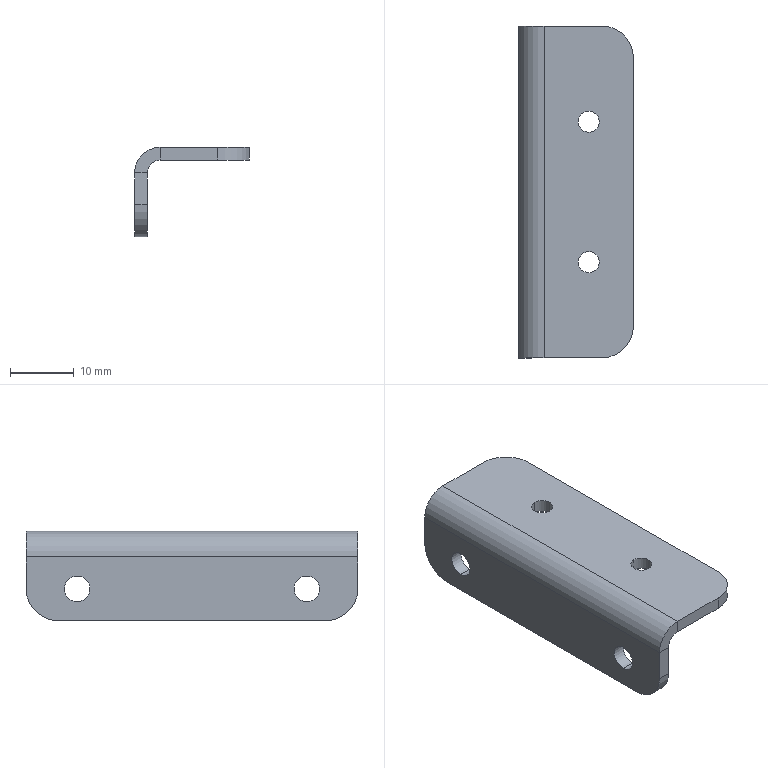Part | NX | features 镜向1 2 | 1 solid | 26 faces | box 18 x 52 x 14 mm | volume 2859 mm3 | cylinder 14 | plane 12 | commonest cylinder face diameters 4 x5 3.3 x4 10 x4 8 x1
STEP:
#1=CARTESIAN_POINT('',(50.,117.,-101.5));
#2=VERTEX_POINT('',#1);
#3=CARTESIAN_POINT('',(50.,117.,-105.5));
#4=VERTEX_POINT('',#3);
#5=CARTESIAN_POINT('',(50.,117.,-103.5));
#6=DIRECTION('',(-1.,0.,0.));
#7=DIRECTION('',(0.,0.,-1.));
#8=AXIS2_PLACEMENT_3D('',#5,#6,#7);
#9=CIRCLE('',#8,2.);
#10=EDGE_CURVE('',#2,#4,#9,.T.);
#11=ORIENTED_EDGE('',*,*,#10,.T.);
#12=CARTESIAN_POINT('',(52.,117.,-105.5));
#13=VERTEX_POINT('',#12);
#14=CARTESIAN_POINT('',(50.,117.,-105.5));
#15=DIRECTION('',(1.,0.,0.));
#16=VECTOR('',#15,1000.);
#17=LINE('',#14,#16);
#18=EDGE_CURVE('',#4,#13,#17,.T.);
#19=ORIENTED_EDGE('',*,*,#18,.T.);
#20=CARTESIAN_POINT('',(52.,117.,-101.5));
#21=VERTEX_POINT('',#20);
#22=CARTESIAN_POINT('',(52.,117.,-103.5));
#23=DIRECTION('',(-1.,0.,0.));
#24=DIRECTION('',(0.,0.,-1.));
#25=AXIS2_PLACEMENT_3D('',#22,#23,#24);
#26=CIRCLE('',#25,2.);
#27=EDGE_CURVE('',#21,#13,#26,.T.);
#28=ORIENTED_EDGE('',*,*,#27,.F.);
#29=CARTESIAN_POINT('',(50.,117.,-101.5));
#30=DIRECTION('',(1.,0.,0.));
#31=VECTOR('',#30,1000.);
#32=LINE('',#29,#31);
#33=EDGE_CURVE('',#21,#2,#32,.F.);
#34=ORIENTED_EDGE('',*,*,#33,.T.);
#35=EDGE_LOOP('',(#11,#19,#28,#34));
#36=FACE_BOUND('',#35,.T.);
#37=CARTESIAN_POINT('',(50.,117.,-103.5));
#38=DIRECTION('',(1.,0.,0.));
#39=DIRECTION('',(0.,0.,-1.));
#40=AXIS2_PLACEMENT_3D('',#37,#38,#39);
#41=CYLINDRICAL_SURFACE('',#40,2.);
#42=ADVANCED_FACE('',(#36),#41,.F.);
#43=CARTESIAN_POINT('',(50.,81.,-101.5));
#44=VERTEX_POINT('',#43);
#45=CARTESIAN_POINT('',(50.,81.,-105.5));
#46=VERTEX_POINT('',#45);
#47=CARTESIAN_POINT('',(50.,81.,-103.5));
#48=DIRECTION('',(-1.,0.,0.));
#49=DIRECTION('',(0.,0.,1.));
#50=AXIS2_PLACEMENT_3D('',#47,#48,#49);
#51=CIRCLE('',#50,2.);
#52=EDGE_CURVE('',#44,#46,#51,.T.);
#53=ORIENTED_EDGE('',*,*,#52,.T.);
#54=CARTESIAN_POINT('',(52.,81.,-105.5));
#55=VERTEX_POINT('',#54);
#56=CARTESIAN_POINT('',(50.,81.,-105.5));
#57=DIRECTION('',(1.,0.,0.));
#58=VECTOR('',#57,1000.);
#59=LINE('',#56,#58);
#60=EDGE_CURVE('',#55,#46,#59,.F.);
#61=ORIENTED_EDGE('',*,*,#60,.F.);
#62=CARTESIAN_POINT('',(52.,81.,-101.5));
#63=VERTEX_POINT('',#62);
#64=CARTESIAN_POINT('',(52.,81.,-103.5));
#65=DIRECTION('',(-1.,0.,0.));
#66=DIRECTION('',(0.,0.,1.));
#67=AXIS2_PLACEMENT_3D('',#64,#65,#66);
#68=CIRCLE('',#67,2.);
#69=EDGE_CURVE('',#63,#55,#68,.T.);
#70=ORIENTED_EDGE('',*,*,#69,.F.);
#71=CARTESIAN_POINT('',(50.,81.,-101.5));
#72=DIRECTION('',(1.,0.,0.));
#73=VECTOR('',#72,1000.);
#74=LINE('',#71,#73);
#75=EDGE_CURVE('',#44,#63,#74,.T.);
#76=ORIENTED_EDGE('',*,*,#75,.F.);
#77=EDGE_LOOP('',(#53,#61,#70,#76));
#78=FACE_BOUND('',#77,.T.);
#79=CARTESIAN_POINT('',(50.,81.,-103.5));
#80=DIRECTION('',(1.,0.,0.));
#81=DIRECTION('',(0.,0.,-1.));
#82=AXIS2_PLACEMENT_3D('',#79,#80,#81);
#83=CYLINDRICAL_SURFACE('',#82,2.);
#84=ADVANCED_FACE('',(#78),#83,.F.);
#85=CARTESIAN_POINT('',(61.,86.35,-96.5));
#86=VERTEX_POINT('',#85);
#87=CARTESIAN_POINT('',(61.,89.65,-96.5));
#88=VERTEX_POINT('',#87);
#89=CARTESIAN_POINT('',(61.,88.,-96.5));
#90=DIRECTION('',(0.,0.,1.));
#91=DIRECTION('',(0.,-1.,0.));
#92=AXIS2_PLACEMENT_3D('',#89,#90,#91);
#93=CIRCLE('',#92,1.65);
#94=EDGE_CURVE('',#86,#88,#93,.T.);
#95=ORIENTED_EDGE('',*,*,#94,.F.);
#96=CARTESIAN_POINT('',(61.,86.35,-94.5));
#97=VERTEX_POINT('',#96);
#98=CARTESIAN_POINT('',(61.,86.35,-94.5));
#99=DIRECTION('',(0.,0.,1.));
#100=VECTOR('',#99,1000.);
#101=LINE('',#98,#100);
#102=EDGE_CURVE('',#97,#86,#101,.F.);
#103=ORIENTED_EDGE('',*,*,#102,.F.);
#104=CARTESIAN_POINT('',(61.,89.65,-94.5));
#105=VERTEX_POINT('',#104);
#106=CARTESIAN_POINT('',(61.,88.,-94.5));
#107=DIRECTION('',(0.,0.,-1.));
#108=DIRECTION('',(0.,1.,0.));
#109=AXIS2_PLACEMENT_3D('',#106,#107,#108);
#110=CIRCLE('',#109,1.65);
#111=EDGE_CURVE('',#105,#97,#110,.T.);
#112=ORIENTED_EDGE('',*,*,#111,.F.);
#113=CARTESIAN_POINT('',(61.,89.65,-94.5));
#114=DIRECTION('',(0.,0.,1.));
#115=VECTOR('',#114,1000.);
#116=LINE('',#113,#115);
#117=EDGE_CURVE('',#88,#105,#116,.T.);
#118=ORIENTED_EDGE('',*,*,#117,.F.);
#119=EDGE_LOOP('',(#95,#103,#112,#118));
#120=FACE_BOUND('',#119,.T.);
#121=CARTESIAN_POINT('',(61.,88.,-94.5));
#122=DIRECTION('',(0.,0.,1.));
#123=DIRECTION('',(0.,-1.,0.));
#124=AXIS2_PLACEMENT_3D('',#121,#122,#123);
#125=CYLINDRICAL_SURFACE('',#124,1.65);
#126=ADVANCED_FACE('',(#120),#125,.F.);
#127=CARTESIAN_POINT('',(61.,108.35,-96.5));
#128=VERTEX_POINT('',#127);
#129=CARTESIAN_POINT('',(61.,111.65,-96.5));
#130=VERTEX_POINT('',#129);
#131=CARTESIAN_POINT('',(61.,110.,-96.5));
#132=DIRECTION('',(0.,0.,1.));
#133=DIRECTION('',(0.,-1.,0.));
#134=AXIS2_PLACEMENT_3D('',#131,#132,#133);
#135=CIRCLE('',#134,1.65);
#136=EDGE_CURVE('',#128,#130,#135,.T.);
#137=ORIENTED_EDGE('',*,*,#136,.F.);
#138=CARTESIAN_POINT('',(61.,108.35,-94.5));
#139=VERTEX_POINT('',#138);
#140=CARTESIAN_POINT('',(61.,108.35,-94.5));
#141=DIRECTION('',(0.,0.,1.));
#142=VECTOR('',#141,1000.);
#143=LINE('',#140,#142);
#144=EDGE_CURVE('',#139,#128,#143,.F.);
#145=ORIENTED_EDGE('',*,*,#144,.F.);
#146=CARTESIAN_POINT('',(61.,111.65,-94.5));
#147=VERTEX_POINT('',#146);
#148=CARTESIAN_POINT('',(61.,110.,-94.5));
#149=DIRECTION('',(0.,0.,-1.));
#150=DIRECTION('',(0.,1.,0.));
#151=AXIS2_PLACEMENT_3D('',#148,#149,#150);
#152=CIRCLE('',#151,1.65);
#153=EDGE_CURVE('',#147,#139,#152,.T.);
#154=ORIENTED_EDGE('',*,*,#153,.F.);
#155=CARTESIAN_POINT('',(61.,111.65,-94.5));
#156=DIRECTION('',(0.,0.,1.));
#157=VECTOR('',#156,1000.);
#158=LINE('',#155,#157);
#159=EDGE_CURVE('',#130,#147,#158,.T.);
#160=ORIENTED_EDGE('',*,*,#159,.F.);
#161=EDGE_LOOP('',(#137,#145,#154,#160));
#162=FACE_BOUND('',#161,.T.);
#163=CARTESIAN_POINT('',(61.,110.,-94.5));
#164=DIRECTION('',(0.,0.,1.));
#165=DIRECTION('',(0.,-1.,0.));
#166=AXIS2_PLACEMENT_3D('',#163,#164,#165);
#167=CYLINDRICAL_SURFACE('',#166,1.65);
#168=ADVANCED_FACE('',(#162),#167,.F.);
#169=ORIENTED_EDGE('',*,*,#111,.T.);
#170=CARTESIAN_POINT('',(61.,88.,-94.5));
#171=DIRECTION('',(0.,0.,-1.));
#172=DIRECTION('',(0.,1.,0.));
#173=AXIS2_PLACEMENT_3D('',#170,#171,#172);
#174=CIRCLE('',#173,1.65);
#175=EDGE_CURVE('',#97,#105,#174,.T.);
#176=ORIENTED_EDGE('',*,*,#175,.T.);
#177=EDGE_LOOP('',(#169,#176));
#178=FACE_BOUND('',#177,.T.);
#179=CARTESIAN_POINT('',(63.,125.,-94.5));
#180=VERTEX_POINT('',#179);
#181=CARTESIAN_POINT('',(54.,125.,-94.5));
#182=VERTEX_POINT('',#181);
#183=CARTESIAN_POINT('',(68.,125.,-94.5));
#184=DIRECTION('',(-1.,0.,0.));
#185=VECTOR('',#184,1000.);
#186=LINE('',#183,#185);
#187=EDGE_CURVE('',#180,#182,#186,.T.);
#188=ORIENTED_EDGE('',*,*,#187,.T.);
#189=CARTESIAN_POINT('',(54.,73.,-94.5));
#190=VERTEX_POINT('',#189);
#191=CARTESIAN_POINT('',(54.,125.,-94.5));
#192=DIRECTION('',(0.,-1.,0.));
#193=VECTOR('',#192,1000.);
#194=LINE('',#191,#193);
#195=EDGE_CURVE('',#182,#190,#194,.T.);
#196=ORIENTED_EDGE('',*,*,#195,.T.);
#197=CARTESIAN_POINT('',(63.,73.,-94.5));
#198=VERTEX_POINT('',#197);
#199=CARTESIAN_POINT('',(68.,73.,-94.5));
#200=DIRECTION('',(-1.,0.,0.));
#201=VECTOR('',#200,1000.);
#202=LINE('',#199,#201);
#203=EDGE_CURVE('',#198,#190,#202,.T.);
#204=ORIENTED_EDGE('',*,*,#203,.F.);
#205=CARTESIAN_POINT('',(68.,78.,-94.5));
#206=VERTEX_POINT('',#205);
#207=CARTESIAN_POINT('',(63.,78.,-94.5));
#208=DIRECTION('',(0.,0.,-1.));
#209=DIRECTION('',(0.,-1.,0.));
#210=AXIS2_PLACEMENT_3D('',#207,#208,#209);
#211=CIRCLE('',#210,5.);
#212=EDGE_CURVE('',#206,#198,#211,.T.);
#213=ORIENTED_EDGE('',*,*,#212,.F.);
#214=CARTESIAN_POINT('',(68.,120.,-94.5));
#215=VERTEX_POINT('',#214);
#216=CARTESIAN_POINT('',(68.,125.,-94.5));
#217=DIRECTION('',(0.,-1.,0.));
#218=VECTOR('',#217,1000.);
#219=LINE('',#216,#218);
#220=EDGE_CURVE('',#215,#206,#219,.T.);
#221=ORIENTED_EDGE('',*,*,#220,.F.);
#222=CARTESIAN_POINT('',(63.,120.,-94.5));
#223=DIRECTION('',(0.,0.,-1.));
#224=DIRECTION('',(0.,-1.,0.));
#225=AXIS2_PLACEMENT_3D('',#222,#223,#224);
#226=CIRCLE('',#225,5.);
#227=EDGE_CURVE('',#180,#215,#226,.T.);
#228=ORIENTED_EDGE('',*,*,#227,.F.);
#229=EDGE_LOOP('',(#188,#196,#204,#213,#221,#228));
#230=FACE_BOUND('',#229,.T.);
#231=ORIENTED_EDGE('',*,*,#153,.T.);
#232=CARTESIAN_POINT('',(61.,110.,-94.5));
#233=DIRECTION('',(0.,0.,-1.));
#234=DIRECTION('',(0.,1.,0.));
#235=AXIS2_PLACEMENT_3D('',#232,#233,#234);
#236=CIRCLE('',#235,1.65);
#237=EDGE_CURVE('',#139,#147,#236,.T.);
#238=ORIENTED_EDGE('',*,*,#237,.T.);
#239=EDGE_LOOP('',(#231,#238));
#240=FACE_BOUND('',#239,.T.);
#241=CARTESIAN_POINT('',(68.,125.,-94.5));
#242=DIRECTION('',(0.,0.,-1.));
#243=DIRECTION('',(0.,1.,0.));
#244=AXIS2_PLACEMENT_3D('',#241,#242,#243);
#245=PLANE('',#244);
#246=ADVANCED_FACE('',(#178,#230,#240),#245,.F.);
#247=CARTESIAN_POINT('',(54.,125.,-96.5));
#248=VERTEX_POINT('',#247);
#249=CARTESIAN_POINT('',(54.,125.,-94.5));
#250=DIRECTION('',(0.,0.,-1.));
#251=VECTOR('',#250,1000.);
#252=LINE('',#249,#251);
#253=EDGE_CURVE('',#182,#248,#252,.T.);
#254=ORIENTED_EDGE('',*,*,#253,.T.);
#255=CARTESIAN_POINT('',(52.,125.,-98.5));
#256=VERTEX_POINT('',#255);
#257=CARTESIAN_POINT('',(54.,125.,-98.5));
#258=DIRECTION('',(0.,-1.,0.));
#259=DIRECTION('',(0.,0.,-1.));
#260=AXIS2_PLACEMENT_3D('',#257,#258,#259);
#261=CIRCLE('',#260,2.);
#262=EDGE_CURVE('',#248,#256,#261,.T.);
#263=ORIENTED_EDGE('',*,*,#262,.T.);
#264=CARTESIAN_POINT('',(50.,125.,-98.5));
#265=VERTEX_POINT('',#264);
#266=CARTESIAN_POINT('',(52.,125.,-98.5));
#267=DIRECTION('',(-1.,0.,0.));
#268=VECTOR('',#267,1000.);
#269=LINE('',#266,#268);
#270=EDGE_CURVE('',#256,#265,#269,.T.);
#271=ORIENTED_EDGE('',*,*,#270,.T.);
#272=CARTESIAN_POINT('',(54.,125.,-98.5));
#273=DIRECTION('',(0.,-1.,0.));
#274=DIRECTION('',(0.,0.,1.));
#275=AXIS2_PLACEMENT_3D('',#272,#273,#274);
#276=CIRCLE('',#275,4.);
#277=EDGE_CURVE('',#182,#265,#276,.T.);
#278=ORIENTED_EDGE('',*,*,#277,.F.);
#279=EDGE_LOOP('',(#254,#263,#271,#278));
#280=FACE_BOUND('',#279,.T.);
#281=CARTESIAN_POINT('',(54.,125.,-94.5));
#282=DIRECTION('',(0.,1.,0.));
#283=DIRECTION('',(0.,0.,1.));
#284=AXIS2_PLACEMENT_3D('',#281,#282,#283);
#285=PLANE('',#284);
#286=ADVANCED_FACE('',(#280),#285,.T.);
#287=CARTESIAN_POINT('',(63.,125.,-96.5));
#288=VERTEX_POINT('',#287);
#289=CARTESIAN_POINT('',(68.,125.,-96.5));
#290=DIRECTION('',(-1.,0.,0.));
#291=VECTOR('',#290,1000.);
#292=LINE('',#289,#291);
#293=EDGE_CURVE('',#288,#248,#292,.T.);
#294=ORIENTED_EDGE('',*,*,#293,.T.);
#295=ORIENTED_EDGE('',*,*,#253,.F.);
#296=ORIENTED_EDGE('',*,*,#187,.F.);
#297=CARTESIAN_POINT('',(63.,125.,-98.5));
#298=DIRECTION('',(0.,0.,1.));
#299=VECTOR('',#298,1000.);
#300=LINE('',#297,#299);
#301=EDGE_CURVE('',#288,#180,#300,.T.);
#302=ORIENTED_EDGE('',*,*,#301,.F.);
#303=EDGE_LOOP('',(#294,#295,#296,#302));
#304=FACE_BOUND('',#303,.T.);
#305=CARTESIAN_POINT('',(52.,125.,-98.5));
#306=DIRECTION('',(0.,1.,0.));
#307=DIRECTION('',(0.,0.,1.));
#308=AXIS2_PLACEMENT_3D('',#305,#306,#307);
#309=PLANE('',#308);
#310=ADVANCED_FACE('',(#304),#309,.T.);
#311=CARTESIAN_POINT('',(50.,73.,-98.5));
#312=VERTEX_POINT('',#311);
#313=CARTESIAN_POINT('',(52.,73.,-98.5));
#314=VERTEX_POINT('',#313);
#315=CARTESIAN_POINT('',(50.,73.,-98.5));
#316=DIRECTION('',(1.,0.,0.));
#317=VECTOR('',#316,1000.);
#318=LINE('',#315,#317);
#319=EDGE_CURVE('',#312,#314,#318,.T.);
#320=ORIENTED_EDGE('',*,*,#319,.T.);
#321=CARTESIAN_POINT('',(54.,73.,-96.5));
#322=VERTEX_POINT('',#321);
#323=CARTESIAN_POINT('',(54.,73.,-98.5));
#324=DIRECTION('',(0.,-1.,0.));
#325=DIRECTION('',(0.,0.,-1.));
#326=AXIS2_PLACEMENT_3D('',#323,#324,#325);
#327=CIRCLE('',#326,2.);
#328=EDGE_CURVE('',#322,#314,#327,.T.);
#329=ORIENTED_EDGE('',*,*,#328,.F.);
#330=CARTESIAN_POINT('',(54.,73.,-96.5));
#331=DIRECTION('',(0.,0.,1.));
#332=VECTOR('',#331,1000.);
#333=LINE('',#330,#332);
#334=EDGE_CURVE('',#322,#190,#333,.T.);
#335=ORIENTED_EDGE('',*,*,#334,.T.);
#336=CARTESIAN_POINT('',(54.,73.,-98.5));
#337=DIRECTION('',(0.,-1.,0.));
#338=DIRECTION('',(0.,0.,1.));
#339=AXIS2_PLACEMENT_3D('',#336,#337,#338);
#340=CIRCLE('',#339,4.);
#341=EDGE_CURVE('',#190,#312,#340,.T.);
#342=ORIENTED_EDGE('',*,*,#341,.T.);
#343=EDGE_LOOP('',(#320,#329,#335,#342));
#344=FACE_BOUND('',#343,.T.);
#345=CARTESIAN_POINT('',(50.,73.,-98.5));
#346=DIRECTION('',(0.,-1.,0.));
#347=DIRECTION('',(0.,0.,-1.));
#348=AXIS2_PLACEMENT_3D('',#345,#346,#347);
#349=PLANE('',#348);
#350=ADVANCED_FACE('',(#344),#349,.T.);
#351=CARTESIAN_POINT('',(52.,73.,-103.5));
#352=VERTEX_POINT('',#351);
#353=CARTESIAN_POINT('',(52.,73.,-94.5));
#354=DIRECTION('',(0.,0.,-1.));
#355=VECTOR('',#354,1000.);
#356=LINE('',#353,#355);
#357=EDGE_CURVE('',#314,#352,#356,.T.);
#358=ORIENTED_EDGE('',*,*,#357,.F.);
#359=ORIENTED_EDGE('',*,*,#319,.F.);
#360=CARTESIAN_POINT('',(50.,73.,-103.5));
#361=VERTEX_POINT('',#360);
#362=CARTESIAN_POINT('',(50.,73.,-94.5));
#363=DIRECTION('',(0.,0.,-1.));
#364=VECTOR('',#363,1000.);
#365=LINE('',#362,#364);
#366=EDGE_CURVE('',#312,#361,#365,.T.);
#367=ORIENTED_EDGE('',*,*,#366,.T.);
#368=CARTESIAN_POINT('',(54.,73.,-103.5));
#369=DIRECTION('',(-1.,0.,0.));
#370=VECTOR('',#369,1000.);
#371=LINE('',#368,#370);
#372=EDGE_CURVE('',#352,#361,#371,.T.);
#373=ORIENTED_EDGE('',*,*,#372,.F.);
#374=EDGE_LOOP('',(#358,#359,#367,#373));
#375=FACE_BOUND('',#374,.T.);
#376=CARTESIAN_POINT('',(54.,73.,-96.5));
#377=DIRECTION('',(0.,-1.,0.));
#378=DIRECTION('',(0.,0.,-1.));
#379=AXIS2_PLACEMENT_3D('',#376,#377,#378);
#380=PLANE('',#379);
#381=ADVANCED_FACE('',(#375),#380,.T.);
#382=ORIENTED_EDGE('',*,*,#10,.F.);
#383=CARTESIAN_POINT('',(50.,117.,-103.5));
#384=DIRECTION('',(-1.,0.,0.));
#385=DIRECTION('',(0.,0.,-1.));
#386=AXIS2_PLACEMENT_3D('',#383,#384,#385);
#387=CIRCLE('',#386,2.);
#388=EDGE_CURVE('',#4,#2,#387,.T.);
#389=ORIENTED_EDGE('',*,*,#388,.F.);
#390=EDGE_LOOP('',(#382,#389));
#391=FACE_BOUND('',#390,.T.);
#392=ORIENTED_EDGE('',*,*,#52,.F.);
#393=CARTESIAN_POINT('',(50.,81.,-103.5));
#394=DIRECTION('',(-1.,0.,0.));
#395=DIRECTION('',(0.,0.,1.));
#396=AXIS2_PLACEMENT_3D('',#393,#394,#395);
#397=CIRCLE('',#396,2.);
#398=EDGE_CURVE('',#46,#44,#397,.T.);
#399=ORIENTED_EDGE('',*,*,#398,.F.);
#400=EDGE_LOOP('',(#392,#399));
#401=FACE_BOUND('',#400,.T.);
#402=CARTESIAN_POINT('',(50.,120.,-108.5));
#403=VERTEX_POINT('',#402);
#404=CARTESIAN_POINT('',(50.,78.,-108.5));
#405=VERTEX_POINT('',#404);
#406=CARTESIAN_POINT('',(50.,125.,-108.5));
#407=DIRECTION('',(0.,-1.,0.));
#408=VECTOR('',#407,1000.);
#409=LINE('',#406,#408);
#410=EDGE_CURVE('',#403,#405,#409,.T.);
#411=ORIENTED_EDGE('',*,*,#410,.T.);
#412=CARTESIAN_POINT('',(50.,78.,-103.5));
#413=DIRECTION('',(1.,0.,0.));
#414=DIRECTION('',(0.,0.,1.));
#415=AXIS2_PLACEMENT_3D('',#412,#413,#414);
#416=CIRCLE('',#415,5.);
#417=EDGE_CURVE('',#361,#405,#416,.T.);
#418=ORIENTED_EDGE('',*,*,#417,.F.);
#419=ORIENTED_EDGE('',*,*,#366,.F.);
#420=CARTESIAN_POINT('',(50.,125.,-98.5));
#421=DIRECTION('',(0.,-1.,0.));
#422=VECTOR('',#421,1000.);
#423=LINE('',#420,#422);
#424=EDGE_CURVE('',#265,#312,#423,.T.);
#425=ORIENTED_EDGE('',*,*,#424,.F.);
#426=CARTESIAN_POINT('',(50.,125.,-103.5));
#427=VERTEX_POINT('',#426);
#428=CARTESIAN_POINT('',(50.,125.,-94.5));
#429=DIRECTION('',(0.,0.,-1.));
#430=VECTOR('',#429,1000.);
#431=LINE('',#428,#430);
#432=EDGE_CURVE('',#265,#427,#431,.T.);
#433=ORIENTED_EDGE('',*,*,#432,.T.);
#434=CARTESIAN_POINT('',(50.,120.,-103.5));
#435=DIRECTION('',(1.,0.,0.));
#436=DIRECTION('',(0.,0.,1.));
#437=AXIS2_PLACEMENT_3D('',#434,#435,#436);
#438=CIRCLE('',#437,5.);
#439=EDGE_CURVE('',#403,#427,#438,.T.);
#440=ORIENTED_EDGE('',*,*,#439,.F.);
#441=EDGE_LOOP('',(#411,#418,#419,#425,#433,#440));
#442=FACE_BOUND('',#441,.T.);
#443=CARTESIAN_POINT('',(50.,125.,-94.5));
#444=DIRECTION('',(1.,0.,0.));
#445=DIRECTION('',(0.,0.,-1.));
#446=AXIS2_PLACEMENT_3D('',#443,#444,#445);
#447=PLANE('',#446);
#448=ADVANCED_FACE('',(#391,#401,#442),#447,.F.);
#449=CARTESIAN_POINT('',(52.,120.,-108.5));
#450=VERTEX_POINT('',#449);
#451=CARTESIAN_POINT('',(52.,78.,-108.5));
#452=VERTEX_POINT('',#451);
#453=CARTESIAN_POINT('',(52.,125.,-108.5));
#454=DIRECTION('',(0.,-1.,0.));
#455=VECTOR('',#454,1000.);
#456=LINE('',#453,#455);
#457=EDGE_CURVE('',#450,#452,#456,.T.);
#458=ORIENTED_EDGE('',*,*,#457,.T.);
#459=CARTESIAN_POINT('',(52.,78.,-108.5));
#460=DIRECTION('',(1.,0.,0.));
#461=VECTOR('',#460,1000.);
#462=LINE('',#459,#461);
#463=EDGE_CURVE('',#405,#452,#462,.T.);
#464=ORIENTED_EDGE('',*,*,#463,.F.);
#465=ORIENTED_EDGE('',*,*,#410,.F.);
#466=CARTESIAN_POINT('',(52.,120.,-108.5));
#467=DIRECTION('',(-1.,0.,0.));
#468=VECTOR('',#467,1000.);
#469=LINE('',#466,#468);
#470=EDGE_CURVE('',#450,#403,#469,.T.);
#471=ORIENTED_EDGE('',*,*,#470,.F.);
#472=EDGE_LOOP('',(#458,#464,#465,#471));
#473=FACE_BOUND('',#472,.T.);
#474=CARTESIAN_POINT('',(52.,125.,-108.5));
#475=DIRECTION('',(0.,0.,-1.));
#476=DIRECTION('',(0.,1.,0.));
#477=AXIS2_PLACEMENT_3D('',#474,#475,#476);
#478=PLANE('',#477);
#479=ADVANCED_FACE('',(#473),#478,.T.);
#480=ORIENTED_EDGE('',*,*,#27,.T.);
#481=CARTESIAN_POINT('',(52.,117.,-103.5));
#482=DIRECTION('',(-1.,0.,0.));
#483=DIRECTION('',(0.,0.,-1.));
#484=AXIS2_PLACEMENT_3D('',#481,#482,#483);
#485=CIRCLE('',#484,2.);
#486=EDGE_CURVE('',#13,#21,#485,.T.);
#487=ORIENTED_EDGE('',*,*,#486,.T.);
#488=EDGE_LOOP('',(#480,#487));
#489=FACE_BOUND('',#488,.T.);
#490=ORIENTED_EDGE('',*,*,#69,.T.);
#491=CARTESIAN_POINT('',(52.,81.,-103.5));
#492=DIRECTION('',(-1.,0.,0.));
#493=DIRECTION('',(0.,0.,1.));
#494=AXIS2_PLACEMENT_3D('',#491,#492,#493);
#495=CIRCLE('',#494,2.);
#496=EDGE_CURVE('',#55,#63,#495,.T.);
#497=ORIENTED_EDGE('',*,*,#496,.T.);
#498=EDGE_LOOP('',(#490,#497));
#499=FACE_BOUND('',#498,.T.);
#500=CARTESIAN_POINT('',(52.,125.,-103.5));
#501=VERTEX_POINT('',#500);
#502=CARTESIAN_POINT('',(52.,125.,-94.5));
#503=DIRECTION('',(0.,0.,-1.));
#504=VECTOR('',#503,1000.);
#505=LINE('',#502,#504);
#506=EDGE_CURVE('',#256,#501,#505,.T.);
#507=ORIENTED_EDGE('',*,*,#506,.F.);
#508=CARTESIAN_POINT('',(52.,125.,-98.5));
#509=DIRECTION('',(0.,-1.,0.));
#510=VECTOR('',#509,1000.);
#511=LINE('',#508,#510);
#512=EDGE_CURVE('',#256,#314,#511,.T.);
#513=ORIENTED_EDGE('',*,*,#512,.T.);
#514=ORIENTED_EDGE('',*,*,#357,.T.);
#515=CARTESIAN_POINT('',(52.,78.,-103.5));
#516=DIRECTION('',(-1.,0.,0.));
#517=DIRECTION('',(0.,0.,1.));
#518=AXIS2_PLACEMENT_3D('',#515,#516,#517);
#519=CIRCLE('',#518,5.);
#520=EDGE_CURVE('',#452,#352,#519,.T.);
#521=ORIENTED_EDGE('',*,*,#520,.F.);
#522=ORIENTED_EDGE('',*,*,#457,.F.);
#523=CARTESIAN_POINT('',(52.,120.,-103.5));
#524=DIRECTION('',(-1.,0.,0.));
#525=DIRECTION('',(0.,0.,1.));
#526=AXIS2_PLACEMENT_3D('',#523,#524,#525);
#527=CIRCLE('',#526,5.);
#528=EDGE_CURVE('',#501,#450,#527,.T.);
#529=ORIENTED_EDGE('',*,*,#528,.F.);
#530=EDGE_LOOP('',(#507,#513,#514,#521,#522,#529));
#531=FACE_BOUND('',#530,.T.);
#532=CARTESIAN_POINT('',(52.,125.,-94.5));
#533=DIRECTION('',(1.,0.,0.));
#534=DIRECTION('',(0.,0.,-1.));
#535=AXIS2_PLACEMENT_3D('',#532,#533,#534);
#536=PLANE('',#535);
#537=ADVANCED_FACE('',(#489,#499,#531),#536,.T.);
#538=ORIENTED_EDGE('',*,*,#328,.T.);
#539=ORIENTED_EDGE('',*,*,#512,.F.);
#540=ORIENTED_EDGE('',*,*,#262,.F.);
#541=CARTESIAN_POINT('',(54.,125.,-96.5));
#542=DIRECTION('',(0.,-1.,0.));
#543=VECTOR('',#542,1000.);
#544=LINE('',#541,#543);
#545=EDGE_CURVE('',#248,#322,#544,.T.);
#546=ORIENTED_EDGE('',*,*,#545,.T.);
#547=EDGE_LOOP('',(#538,#539,#540,#546));
#548=FACE_BOUND('',#547,.T.);
#549=CARTESIAN_POINT('',(54.,125.,-98.5));
#550=DIRECTION('',(0.,-1.,0.));
#551=DIRECTION('',(0.,0.,-1.));
#552=AXIS2_PLACEMENT_3D('',#549,#550,#551);
#553=CYLINDRICAL_SURFACE('',#552,2.);
#554=ADVANCED_FACE('',(#548),#553,.F.);
#555=CARTESIAN_POINT('',(61.,88.,-96.5));
#556=DIRECTION('',(0.,0.,1.));
#557=DIRECTION('',(0.,-1.,0.));
#558=AXIS2_PLACEMENT_3D('',#555,#556,#557);
#559=CIRCLE('',#558,1.65);
#560=EDGE_CURVE('',#88,#86,#559,.T.);
#561=ORIENTED_EDGE('',*,*,#560,.T.);
#562=ORIENTED_EDGE('',*,*,#94,.T.);
#563=EDGE_LOOP('',(#561,#562));
#564=FACE_BOUND('',#563,.T.);
#565=CARTESIAN_POINT('',(61.,110.,-96.5));
#566=DIRECTION('',(0.,0.,1.));
#567=DIRECTION('',(0.,-1.,0.));
#568=AXIS2_PLACEMENT_3D('',#565,#566,#567);
#569=CIRCLE('',#568,1.65);
#570=EDGE_CURVE('',#130,#128,#569,.T.);
#571=ORIENTED_EDGE('',*,*,#570,.T.);
#572=ORIENTED_EDGE('',*,*,#136,.T.);
#573=EDGE_LOOP('',(#571,#572));
#574=FACE_BOUND('',#573,.T.);
#575=CARTESIAN_POINT('',(68.,120.,-96.5));
#576=VERTEX_POINT('',#575);
#577=CARTESIAN_POINT('',(68.,78.,-96.5));
#578=VERTEX_POINT('',#577);
#579=CARTESIAN_POINT('',(68.,125.,-96.5));
#580=DIRECTION('',(0.,-1.,0.));
#581=VECTOR('',#580,1000.);
#582=LINE('',#579,#581);
#583=EDGE_CURVE('',#576,#578,#582,.T.);
#584=ORIENTED_EDGE('',*,*,#583,.T.);
#585=CARTESIAN_POINT('',(63.,73.,-96.5));
#586=VERTEX_POINT('',#585);
#587=CARTESIAN_POINT('',(63.,78.,-96.5));
#588=DIRECTION('',(0.,0.,1.));
#589=DIRECTION('',(0.,-1.,0.));
#590=AXIS2_PLACEMENT_3D('',#587,#588,#589);
#591=CIRCLE('',#590,5.);
#592=EDGE_CURVE('',#586,#578,#591,.T.);
#593=ORIENTED_EDGE('',*,*,#592,.F.);
#594=CARTESIAN_POINT('',(68.,73.,-96.5));
#595=DIRECTION('',(-1.,0.,0.));
#596=VECTOR('',#595,1000.);
#597=LINE('',#594,#596);
#598=EDGE_CURVE('',#586,#322,#597,.T.);
#599=ORIENTED_EDGE('',*,*,#598,.T.);
#600=ORIENTED_EDGE('',*,*,#545,.F.);
#601=ORIENTED_EDGE('',*,*,#293,.F.);
#602=CARTESIAN_POINT('',(63.,120.,-96.5));
#603=DIRECTION('',(0.,0.,1.));
#604=DIRECTION('',(0.,-1.,0.));
#605=AXIS2_PLACEMENT_3D('',#602,#603,#604);
#606=CIRCLE('',#605,5.);
#607=EDGE_CURVE('',#576,#288,#606,.T.);
#608=ORIENTED_EDGE('',*,*,#607,.F.);
#609=EDGE_LOOP('',(#584,#593,#599,#600,#601,#608));
#610=FACE_BOUND('',#609,.T.);
#611=CARTESIAN_POINT('',(68.,125.,-96.5));
#612=DIRECTION('',(0.,0.,-1.));
#613=DIRECTION('',(0.,1.,0.));
#614=AXIS2_PLACEMENT_3D('',#611,#612,#613);
#615=PLANE('',#614);
#616=ADVANCED_FACE('',(#564,#574,#610),#615,.T.);
#617=ORIENTED_EDGE('',*,*,#220,.T.);
#618=CARTESIAN_POINT('',(68.,78.,-94.5));
#619=DIRECTION('',(0.,0.,1.));
#620=VECTOR('',#619,1000.);
#621=LINE('',#618,#620);
#622=EDGE_CURVE('',#578,#206,#621,.T.);
#623=ORIENTED_EDGE('',*,*,#622,.F.);
#624=ORIENTED_EDGE('',*,*,#583,.F.);
#625=CARTESIAN_POINT('',(68.,120.,-94.5));
#626=DIRECTION('',(0.,0.,-1.));
#627=VECTOR('',#626,1000.);
#628=LINE('',#625,#627);
#629=EDGE_CURVE('',#215,#576,#628,.T.);
#630=ORIENTED_EDGE('',*,*,#629,.F.);
#631=EDGE_LOOP('',(#617,#623,#624,#630));
#632=FACE_BOUND('',#631,.T.);
#633=CARTESIAN_POINT('',(68.,125.,-94.5));
#634=DIRECTION('',(1.,0.,0.));
#635=DIRECTION('',(0.,-1.,0.));
#636=AXIS2_PLACEMENT_3D('',#633,#634,#635);
#637=PLANE('',#636);
#638=ADVANCED_FACE('',(#632),#637,.T.);
#639=ORIENTED_EDGE('',*,*,#341,.F.);
#640=ORIENTED_EDGE('',*,*,#195,.F.);
#641=ORIENTED_EDGE('',*,*,#277,.T.);
#642=ORIENTED_EDGE('',*,*,#424,.T.);
#643=EDGE_LOOP('',(#639,#640,#641,#642));
#644=FACE_BOUND('',#643,.T.);
#645=CARTESIAN_POINT('',(54.,125.,-98.5));
#646=DIRECTION('',(0.,-1.,0.));
#647=DIRECTION('',(0.,0.,-1.));
#648=AXIS2_PLACEMENT_3D('',#645,#646,#647);
#649=CYLINDRICAL_SURFACE('',#648,4.);
#650=ADVANCED_FACE('',(#644),#649,.T.);
#651=ORIENTED_EDGE('',*,*,#432,.F.);
#652=ORIENTED_EDGE('',*,*,#270,.F.);
#653=ORIENTED_EDGE('',*,*,#506,.T.);
#654=CARTESIAN_POINT('',(54.,125.,-103.5));
#655=DIRECTION('',(1.,0.,0.));
#656=VECTOR('',#655,1000.);
#657=LINE('',#654,#656);
#658=EDGE_CURVE('',#427,#501,#657,.T.);
#659=ORIENTED_EDGE('',*,*,#658,.F.);
#660=EDGE_LOOP('',(#651,#652,#653,#659));
#661=FACE_BOUND('',#660,.T.);
#662=CARTESIAN_POINT('',(54.,125.,-98.5));
#663=DIRECTION('',(0.,1.,0.));
#664=DIRECTION('',(0.,0.,1.));
#665=AXIS2_PLACEMENT_3D('',#662,#663,#664);
#666=PLANE('',#665);
#667=ADVANCED_FACE('',(#661),#666,.T.);
#668=ORIENTED_EDGE('',*,*,#203,.T.);
#669=ORIENTED_EDGE('',*,*,#334,.F.);
#670=ORIENTED_EDGE('',*,*,#598,.F.);
#671=CARTESIAN_POINT('',(63.,73.,-96.5));
#672=DIRECTION('',(0.,0.,-1.));
#673=VECTOR('',#672,1000.);
#674=LINE('',#671,#673);
#675=EDGE_CURVE('',#198,#586,#674,.T.);
#676=ORIENTED_EDGE('',*,*,#675,.F.);
#677=EDGE_LOOP('',(#668,#669,#670,#676));
#678=FACE_BOUND('',#677,.T.);
#679=CARTESIAN_POINT('',(54.,73.,-98.5));
#680=DIRECTION('',(0.,1.,0.));
#681=DIRECTION('',(0.,0.,1.));
#682=AXIS2_PLACEMENT_3D('',#679,#680,#681);
#683=PLANE('',#682);
#684=ADVANCED_FACE('',(#678),#683,.F.);
#685=ORIENTED_EDGE('',*,*,#144,.T.);
#686=ORIENTED_EDGE('',*,*,#570,.F.);
#687=ORIENTED_EDGE('',*,*,#159,.T.);
#688=ORIENTED_EDGE('',*,*,#237,.F.);
#689=EDGE_LOOP('',(#685,#686,#687,#688));
#690=FACE_BOUND('',#689,.T.);
#691=CARTESIAN_POINT('',(61.,110.,-94.5));
#692=DIRECTION('',(0.,0.,1.));
#693=DIRECTION('',(0.,-1.,0.));
#694=AXIS2_PLACEMENT_3D('',#691,#692,#693);
#695=CYLINDRICAL_SURFACE('',#694,1.65);
#696=ADVANCED_FACE('',(#690),#695,.F.);
#697=ORIENTED_EDGE('',*,*,#102,.T.);
#698=ORIENTED_EDGE('',*,*,#560,.F.);
#699=ORIENTED_EDGE('',*,*,#117,.T.);
#700=ORIENTED_EDGE('',*,*,#175,.F.);
#701=EDGE_LOOP('',(#697,#698,#699,#700));
#702=FACE_BOUND('',#701,.T.);
#703=CARTESIAN_POINT('',(61.,88.,-94.5));
#704=DIRECTION('',(0.,0.,1.));
#705=DIRECTION('',(0.,-1.,0.));
#706=AXIS2_PLACEMENT_3D('',#703,#704,#705);
#707=CYLINDRICAL_SURFACE('',#706,1.65);
#708=ADVANCED_FACE('',(#702),#707,.F.);
#709=ORIENTED_EDGE('',*,*,#528,.T.);
#710=ORIENTED_EDGE('',*,*,#470,.T.);
#711=ORIENTED_EDGE('',*,*,#439,.T.);
#712=ORIENTED_EDGE('',*,*,#658,.T.);
#713=EDGE_LOOP('',(#709,#710,#711,#712));
#714=FACE_BOUND('',#713,.T.);
#715=CARTESIAN_POINT('',(52.,120.,-103.5));
#716=DIRECTION('',(-1.,0.,0.));
#717=DIRECTION('',(0.,1.,0.));
#718=AXIS2_PLACEMENT_3D('',#715,#716,#717);
#719=CYLINDRICAL_SURFACE('',#718,5.);
#720=ADVANCED_FACE('',(#714),#719,.T.);
#721=ORIENTED_EDGE('',*,*,#520,.T.);
#722=ORIENTED_EDGE('',*,*,#372,.T.);
#723=ORIENTED_EDGE('',*,*,#417,.T.);
#724=ORIENTED_EDGE('',*,*,#463,.T.);
#725=EDGE_LOOP('',(#721,#722,#723,#724));
#726=FACE_BOUND('',#725,.T.);
#727=CARTESIAN_POINT('',(54.,78.,-103.5));
#728=DIRECTION('',(-1.,0.,0.));
#729=DIRECTION('',(0.,1.,0.));
#730=AXIS2_PLACEMENT_3D('',#727,#728,#729);
#731=CYLINDRICAL_SURFACE('',#730,5.);
#732=ADVANCED_FACE('',(#726),#731,.T.);
#733=ORIENTED_EDGE('',*,*,#227,.T.);
#734=ORIENTED_EDGE('',*,*,#629,.T.);
#735=ORIENTED_EDGE('',*,*,#607,.T.);
#736=ORIENTED_EDGE('',*,*,#301,.T.);
#737=EDGE_LOOP('',(#733,#734,#735,#736));
#738=FACE_BOUND('',#737,.T.);
#739=CARTESIAN_POINT('',(63.,120.,-94.5));
#740=DIRECTION('',(0.,0.,-1.));
#741=DIRECTION('',(0.,1.,0.));
#742=AXIS2_PLACEMENT_3D('',#739,#740,#741);
#743=CYLINDRICAL_SURFACE('',#742,5.);
#744=ADVANCED_FACE('',(#738),#743,.T.);
#745=ORIENTED_EDGE('',*,*,#212,.T.);
#746=ORIENTED_EDGE('',*,*,#675,.T.);
#747=ORIENTED_EDGE('',*,*,#592,.T.);
#748=ORIENTED_EDGE('',*,*,#622,.T.);
#749=EDGE_LOOP('',(#745,#746,#747,#748));
#750=FACE_BOUND('',#749,.T.);
#751=CARTESIAN_POINT('',(63.,78.,-98.5));
#752=DIRECTION('',(0.,0.,1.));
#753=DIRECTION('',(0.,-1.,0.));
#754=AXIS2_PLACEMENT_3D('',#751,#752,#753);
#755=CYLINDRICAL_SURFACE('',#754,5.);
#756=ADVANCED_FACE('',(#750),#755,.T.);
#757=ORIENTED_EDGE('',*,*,#60,.T.);
#758=ORIENTED_EDGE('',*,*,#398,.T.);
#759=ORIENTED_EDGE('',*,*,#75,.T.);
#760=ORIENTED_EDGE('',*,*,#496,.F.);
#761=EDGE_LOOP('',(#757,#758,#759,#760));
#762=FACE_BOUND('',#761,.T.);
#763=CARTESIAN_POINT('',(50.,81.,-103.5));
#764=DIRECTION('',(1.,0.,0.));
#765=DIRECTION('',(0.,0.,-1.));
#766=AXIS2_PLACEMENT_3D('',#763,#764,#765);
#767=CYLINDRICAL_SURFACE('',#766,2.);
#768=ADVANCED_FACE('',(#762),#767,.F.);
#769=ORIENTED_EDGE('',*,*,#18,.F.);
#770=ORIENTED_EDGE('',*,*,#388,.T.);
#771=ORIENTED_EDGE('',*,*,#33,.F.);
#772=ORIENTED_EDGE('',*,*,#486,.F.);
#773=EDGE_LOOP('',(#769,#770,#771,#772));
#774=FACE_BOUND('',#773,.T.);
#775=CARTESIAN_POINT('',(50.,117.,-103.5));
#776=DIRECTION('',(1.,0.,0.));
#777=DIRECTION('',(0.,0.,-1.));
#778=AXIS2_PLACEMENT_3D('',#775,#776,#777);
#779=CYLINDRICAL_SURFACE('',#778,2.);
#780=ADVANCED_FACE('',(#774),#779,.F.);
#781=CLOSED_SHELL('',(#42,#84,#126,#168,#246,#286,#310,#350,#381,#448,#479,#537,#554,#616,#638,#650,#667,#684,#696,#708,#720,#732,#744,#756,#768,#780));
#782=MANIFOLD_SOLID_BREP('',#781);
#783=(LENGTH_UNIT()NAMED_UNIT(*)SI_UNIT(.MILLI.,.METRE.));
#784=UNCERTAINTY_MEASURE_WITH_UNIT(LENGTH_MEASURE(0.00001),#783,'','');
#785=(NAMED_UNIT(*)PLANE_ANGLE_UNIT()SI_UNIT($,.RADIAN.));
#786=(NAMED_UNIT(*)SI_UNIT($,.STERADIAN.)SOLID_ANGLE_UNIT());
#787=(GEOMETRIC_REPRESENTATION_CONTEXT(3)GLOBAL_UNCERTAINTY_ASSIGNED_CONTEXT((#784))GLOBAL_UNIT_ASSIGNED_CONTEXT((#783,#785,#786))REPRESENTATION_CONTEXT('',''));
#788=ADVANCED_BREP_SHAPE_REPRESENTATION('',(#782),#787);